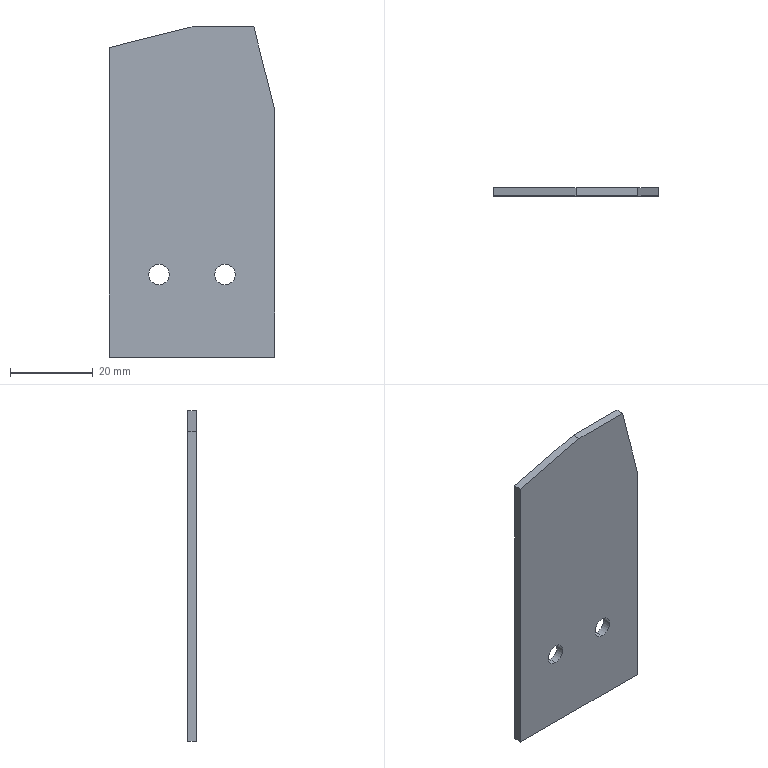Part | SolidWorks | features Chamfer 1, Cut 1, Extrusion 1 | 1 solid | 12 faces | box 40 x 2 x 80 mm | volume 6121 mm3 | plane 8 | cylinder 4 | commonest cylinder face diameters 5 x4
STEP:
#1=CARTESIAN_POINT('',(8.,2.,-22.5));
#2=VERTEX_POINT('',#1);
#3=CARTESIAN_POINT('',(8.,2.,-17.5));
#4=VERTEX_POINT('',#3);
#5=CARTESIAN_POINT('',(8.,2.,-20.));
#6=DIRECTION('',(0.,1.,0.));
#7=DIRECTION('',(0.,0.,1.));
#8=AXIS2_PLACEMENT_3D('',#5,#6,#7);
#9=CIRCLE('',#8,2.5);
#10=EDGE_CURVE('',#2,#4,#9,.T.);
#11=ORIENTED_EDGE('',*,*,#10,.T.);
#12=CARTESIAN_POINT('',(8.,0.,-17.5));
#13=VERTEX_POINT('',#12);
#14=CARTESIAN_POINT('',(8.,10.,-17.5));
#15=DIRECTION('',(0.,-1.,0.));
#16=VECTOR('',#15,1000.);
#17=LINE('',#14,#16);
#18=EDGE_CURVE('',#4,#13,#17,.T.);
#19=ORIENTED_EDGE('',*,*,#18,.T.);
#20=CARTESIAN_POINT('',(8.,0.,-22.5));
#21=VERTEX_POINT('',#20);
#22=CARTESIAN_POINT('',(8.,0.,-20.));
#23=DIRECTION('',(0.,-1.,0.));
#24=DIRECTION('',(0.,0.,-1.));
#25=AXIS2_PLACEMENT_3D('',#22,#23,#24);
#26=CIRCLE('',#25,2.5);
#27=EDGE_CURVE('',#13,#21,#26,.T.);
#28=ORIENTED_EDGE('',*,*,#27,.T.);
#29=CARTESIAN_POINT('',(8.,10.,-22.5));
#30=DIRECTION('',(0.,-1.,0.));
#31=VECTOR('',#30,1000.);
#32=LINE('',#29,#31);
#33=EDGE_CURVE('',#2,#21,#32,.T.);
#34=ORIENTED_EDGE('',*,*,#33,.F.);
#35=EDGE_LOOP('',(#11,#19,#28,#34));
#36=FACE_OUTER_BOUND('',#35,.T.);
#37=CARTESIAN_POINT('',(8.,10.,-20.));
#38=DIRECTION('',(0.,-1.,0.));
#39=DIRECTION('',(0.,0.,-1.));
#40=AXIS2_PLACEMENT_3D('',#37,#38,#39);
#41=CYLINDRICAL_SURFACE('',#40,2.5);
#42=ADVANCED_FACE('',(#36),#41,.F.);
#43=CARTESIAN_POINT('',(-8.,2.,-22.5));
#44=VERTEX_POINT('',#43);
#45=CARTESIAN_POINT('',(-8.,2.,-17.5));
#46=VERTEX_POINT('',#45);
#47=CARTESIAN_POINT('',(-8.,2.,-20.));
#48=DIRECTION('',(0.,1.,0.));
#49=DIRECTION('',(0.,0.,1.));
#50=AXIS2_PLACEMENT_3D('',#47,#48,#49);
#51=CIRCLE('',#50,2.5);
#52=EDGE_CURVE('',#44,#46,#51,.T.);
#53=ORIENTED_EDGE('',*,*,#52,.T.);
#54=CARTESIAN_POINT('',(-8.,0.,-17.5));
#55=VERTEX_POINT('',#54);
#56=CARTESIAN_POINT('',(-8.,10.,-17.5));
#57=DIRECTION('',(0.,-1.,0.));
#58=VECTOR('',#57,1000.);
#59=LINE('',#56,#58);
#60=EDGE_CURVE('',#46,#55,#59,.T.);
#61=ORIENTED_EDGE('',*,*,#60,.T.);
#62=CARTESIAN_POINT('',(-8.,0.,-22.5));
#63=VERTEX_POINT('',#62);
#64=CARTESIAN_POINT('',(-8.,0.,-20.));
#65=DIRECTION('',(0.,-1.,0.));
#66=DIRECTION('',(0.,0.,-1.));
#67=AXIS2_PLACEMENT_3D('',#64,#65,#66);
#68=CIRCLE('',#67,2.5);
#69=EDGE_CURVE('',#55,#63,#68,.T.);
#70=ORIENTED_EDGE('',*,*,#69,.T.);
#71=CARTESIAN_POINT('',(-8.,10.,-22.5));
#72=DIRECTION('',(0.,-1.,0.));
#73=VECTOR('',#72,1000.);
#74=LINE('',#71,#73);
#75=EDGE_CURVE('',#44,#63,#74,.T.);
#76=ORIENTED_EDGE('',*,*,#75,.F.);
#77=EDGE_LOOP('',(#53,#61,#70,#76));
#78=FACE_OUTER_BOUND('',#77,.T.);
#79=CARTESIAN_POINT('',(-8.,10.,-20.));
#80=DIRECTION('',(0.,-1.,0.));
#81=DIRECTION('',(0.,0.,-1.));
#82=AXIS2_PLACEMENT_3D('',#79,#80,#81);
#83=CYLINDRICAL_SURFACE('',#82,2.5);
#84=ADVANCED_FACE('',(#78),#83,.F.);
#85=CARTESIAN_POINT('',(20.,2.,20.));
#86=VERTEX_POINT('',#85);
#87=CARTESIAN_POINT('',(20.,2.,-40.));
#88=VERTEX_POINT('',#87);
#89=CARTESIAN_POINT('',(20.,2.,-40.));
#90=DIRECTION('',(0.,0.,-1.));
#91=VECTOR('',#90,1000.);
#92=LINE('',#89,#91);
#93=EDGE_CURVE('',#86,#88,#92,.T.);
#94=ORIENTED_EDGE('',*,*,#93,.F.);
#95=CARTESIAN_POINT('',(20.,0.,20.));
#96=VERTEX_POINT('',#95);
#97=CARTESIAN_POINT('',(20.,2.,20.));
#98=DIRECTION('',(0.,-1.,0.));
#99=VECTOR('',#98,1000.);
#100=LINE('',#97,#99);
#101=EDGE_CURVE('',#86,#96,#100,.T.);
#102=ORIENTED_EDGE('',*,*,#101,.T.);
#103=CARTESIAN_POINT('',(20.,0.,-40.));
#104=VERTEX_POINT('',#103);
#105=CARTESIAN_POINT('',(20.,0.,-40.));
#106=DIRECTION('',(0.,0.,-1.));
#107=VECTOR('',#106,1000.);
#108=LINE('',#105,#107);
#109=EDGE_CURVE('',#96,#104,#108,.T.);
#110=ORIENTED_EDGE('',*,*,#109,.T.);
#111=CARTESIAN_POINT('',(20.,2.,-40.));
#112=DIRECTION('',(0.,-1.,0.));
#113=VECTOR('',#112,1000.);
#114=LINE('',#111,#113);
#115=EDGE_CURVE('',#88,#104,#114,.T.);
#116=ORIENTED_EDGE('',*,*,#115,.F.);
#117=EDGE_LOOP('',(#94,#102,#110,#116));
#118=FACE_OUTER_BOUND('',#117,.T.);
#119=CARTESIAN_POINT('',(20.,2.,-40.));
#120=DIRECTION('',(-1.,0.,0.));
#121=DIRECTION('',(0.,0.,1.));
#122=AXIS2_PLACEMENT_3D('',#119,#120,#121);
#123=PLANE('',#122);
#124=ADVANCED_FACE('',(#118),#123,.F.);
#125=CARTESIAN_POINT('',(-20.,0.,-40.));
#126=VERTEX_POINT('',#125);
#127=CARTESIAN_POINT('',(-20.,0.,-40.));
#128=DIRECTION('',(-1.,0.,0.));
#129=VECTOR('',#128,1000.);
#130=LINE('',#127,#129);
#131=EDGE_CURVE('',#104,#126,#130,.T.);
#132=ORIENTED_EDGE('',*,*,#131,.T.);
#133=CARTESIAN_POINT('',(-20.,2.,-40.));
#134=VERTEX_POINT('',#133);
#135=CARTESIAN_POINT('',(-20.,2.,-40.));
#136=DIRECTION('',(0.,-1.,0.));
#137=VECTOR('',#136,1000.);
#138=LINE('',#135,#137);
#139=EDGE_CURVE('',#134,#126,#138,.T.);
#140=ORIENTED_EDGE('',*,*,#139,.F.);
#141=CARTESIAN_POINT('',(-20.,2.,-40.));
#142=DIRECTION('',(-1.,0.,0.));
#143=VECTOR('',#142,1000.);
#144=LINE('',#141,#143);
#145=EDGE_CURVE('',#88,#134,#144,.T.);
#146=ORIENTED_EDGE('',*,*,#145,.F.);
#147=ORIENTED_EDGE('',*,*,#115,.T.);
#148=EDGE_LOOP('',(#132,#140,#146,#147));
#149=FACE_OUTER_BOUND('',#148,.T.);
#150=CARTESIAN_POINT('',(-20.,2.,-40.));
#151=DIRECTION('',(0.,0.,1.));
#152=DIRECTION('',(1.,0.,0.));
#153=AXIS2_PLACEMENT_3D('',#150,#151,#152);
#154=PLANE('',#153);
#155=ADVANCED_FACE('',(#149),#154,.F.);
#156=CARTESIAN_POINT('',(-20.,0.,35.));
#157=VERTEX_POINT('',#156);
#158=CARTESIAN_POINT('',(-20.,0.,-40.));
#159=DIRECTION('',(0.,0.,1.));
#160=VECTOR('',#159,1000.);
#161=LINE('',#158,#160);
#162=EDGE_CURVE('',#126,#157,#161,.T.);
#163=ORIENTED_EDGE('',*,*,#162,.T.);
#164=CARTESIAN_POINT('',(-20.,2.,35.));
#165=VERTEX_POINT('',#164);
#166=CARTESIAN_POINT('',(-20.,2.,35.));
#167=DIRECTION('',(0.,1.,0.));
#168=VECTOR('',#167,1000.);
#169=LINE('',#166,#168);
#170=EDGE_CURVE('',#157,#165,#169,.T.);
#171=ORIENTED_EDGE('',*,*,#170,.T.);
#172=CARTESIAN_POINT('',(-20.,2.,-40.));
#173=DIRECTION('',(0.,0.,1.));
#174=VECTOR('',#173,1000.);
#175=LINE('',#172,#174);
#176=EDGE_CURVE('',#134,#165,#175,.T.);
#177=ORIENTED_EDGE('',*,*,#176,.F.);
#178=ORIENTED_EDGE('',*,*,#139,.T.);
#179=EDGE_LOOP('',(#163,#171,#177,#178));
#180=FACE_OUTER_BOUND('',#179,.T.);
#181=CARTESIAN_POINT('',(-20.,2.,-40.));
#182=DIRECTION('',(1.,0.,0.));
#183=DIRECTION('',(0.,0.,-1.));
#184=AXIS2_PLACEMENT_3D('',#181,#182,#183);
#185=PLANE('',#184);
#186=ADVANCED_FACE('',(#180),#185,.F.);
#187=CARTESIAN_POINT('',(0.,0.,40.));
#188=VERTEX_POINT('',#187);
#189=CARTESIAN_POINT('',(15.,0.,40.));
#190=VERTEX_POINT('',#189);
#191=CARTESIAN_POINT('',(-20.,0.,40.));
#192=DIRECTION('',(1.,0.,0.));
#193=VECTOR('',#192,1000.);
#194=LINE('',#191,#193);
#195=EDGE_CURVE('',#188,#190,#194,.T.);
#196=ORIENTED_EDGE('',*,*,#195,.T.);
#197=CARTESIAN_POINT('',(15.,2.,40.));
#198=VERTEX_POINT('',#197);
#199=CARTESIAN_POINT('',(15.,2.,40.));
#200=DIRECTION('',(0.,1.,0.));
#201=VECTOR('',#200,1000.);
#202=LINE('',#199,#201);
#203=EDGE_CURVE('',#190,#198,#202,.T.);
#204=ORIENTED_EDGE('',*,*,#203,.T.);
#205=CARTESIAN_POINT('',(0.,2.,40.));
#206=VERTEX_POINT('',#205);
#207=CARTESIAN_POINT('',(-20.,2.,40.));
#208=DIRECTION('',(1.,0.,0.));
#209=VECTOR('',#208,1000.);
#210=LINE('',#207,#209);
#211=EDGE_CURVE('',#206,#198,#210,.T.);
#212=ORIENTED_EDGE('',*,*,#211,.F.);
#213=CARTESIAN_POINT('',(0.,2.,40.));
#214=DIRECTION('',(0.,-1.,0.));
#215=VECTOR('',#214,1000.);
#216=LINE('',#213,#215);
#217=EDGE_CURVE('',#206,#188,#216,.T.);
#218=ORIENTED_EDGE('',*,*,#217,.T.);
#219=EDGE_LOOP('',(#196,#204,#212,#218));
#220=FACE_OUTER_BOUND('',#219,.T.);
#221=CARTESIAN_POINT('',(-20.,2.,40.));
#222=DIRECTION('',(0.,0.,-1.));
#223=DIRECTION('',(-1.,0.,0.));
#224=AXIS2_PLACEMENT_3D('',#221,#222,#223);
#225=PLANE('',#224);
#226=ADVANCED_FACE('',(#220),#225,.F.);
#227=ORIENTED_EDGE('',*,*,#10,.F.);
#228=CARTESIAN_POINT('',(8.,2.,-20.));
#229=DIRECTION('',(0.,1.,0.));
#230=DIRECTION('',(0.,0.,1.));
#231=AXIS2_PLACEMENT_3D('',#228,#229,#230);
#232=CIRCLE('',#231,2.5);
#233=EDGE_CURVE('',#4,#2,#232,.T.);
#234=ORIENTED_EDGE('',*,*,#233,.F.);
#235=EDGE_LOOP('',(#227,#234));
#236=FACE_BOUND('',#235,.T.);
#237=ORIENTED_EDGE('',*,*,#52,.F.);
#238=CARTESIAN_POINT('',(-8.,2.,-20.));
#239=DIRECTION('',(0.,1.,0.));
#240=DIRECTION('',(0.,0.,1.));
#241=AXIS2_PLACEMENT_3D('',#238,#239,#240);
#242=CIRCLE('',#241,2.5);
#243=EDGE_CURVE('',#46,#44,#242,.T.);
#244=ORIENTED_EDGE('',*,*,#243,.F.);
#245=EDGE_LOOP('',(#237,#244));
#246=FACE_BOUND('',#245,.T.);
#247=ORIENTED_EDGE('',*,*,#211,.T.);
#248=CARTESIAN_POINT('',(23.529,2.,5.882));
#249=DIRECTION('',(0.2425,0.,-0.9701));
#250=VECTOR('',#249,1000.);
#251=LINE('',#248,#250);
#252=EDGE_CURVE('',#198,#86,#251,.T.);
#253=ORIENTED_EDGE('',*,*,#252,.T.);
#254=ORIENTED_EDGE('',*,*,#93,.T.);
#255=ORIENTED_EDGE('',*,*,#145,.T.);
#256=ORIENTED_EDGE('',*,*,#176,.T.);
#257=CARTESIAN_POINT('',(-9.412,2.,37.647));
#258=DIRECTION('',(0.9701,0.,0.2425));
#259=VECTOR('',#258,1000.);
#260=LINE('',#257,#259);
#261=EDGE_CURVE('',#165,#206,#260,.T.);
#262=ORIENTED_EDGE('',*,*,#261,.T.);
#263=EDGE_LOOP('',(#247,#253,#254,#255,#256,#262));
#264=FACE_OUTER_BOUND('',#263,.T.);
#265=CARTESIAN_POINT('',(0.,2.,0.));
#266=DIRECTION('',(0.,1.,0.));
#267=DIRECTION('',(0.,0.,1.));
#268=AXIS2_PLACEMENT_3D('',#265,#266,#267);
#269=PLANE('',#268);
#270=ADVANCED_FACE('',(#236,#246,#264),#269,.T.);
#271=CARTESIAN_POINT('',(8.,0.,-20.));
#272=DIRECTION('',(0.,-1.,0.));
#273=DIRECTION('',(0.,0.,-1.));
#274=AXIS2_PLACEMENT_3D('',#271,#272,#273);
#275=CIRCLE('',#274,2.5);
#276=EDGE_CURVE('',#21,#13,#275,.T.);
#277=ORIENTED_EDGE('',*,*,#276,.F.);
#278=ORIENTED_EDGE('',*,*,#27,.F.);
#279=EDGE_LOOP('',(#277,#278));
#280=FACE_BOUND('',#279,.T.);
#281=CARTESIAN_POINT('',(-8.,0.,-20.));
#282=DIRECTION('',(0.,-1.,0.));
#283=DIRECTION('',(0.,0.,-1.));
#284=AXIS2_PLACEMENT_3D('',#281,#282,#283);
#285=CIRCLE('',#284,2.5);
#286=EDGE_CURVE('',#63,#55,#285,.T.);
#287=ORIENTED_EDGE('',*,*,#286,.F.);
#288=ORIENTED_EDGE('',*,*,#69,.F.);
#289=EDGE_LOOP('',(#287,#288));
#290=FACE_BOUND('',#289,.T.);
#291=ORIENTED_EDGE('',*,*,#109,.F.);
#292=CARTESIAN_POINT('',(20.,0.,20.));
#293=DIRECTION('',(-0.2425,0.,0.9701));
#294=VECTOR('',#293,1000.);
#295=LINE('',#292,#294);
#296=EDGE_CURVE('',#96,#190,#295,.T.);
#297=ORIENTED_EDGE('',*,*,#296,.T.);
#298=ORIENTED_EDGE('',*,*,#195,.F.);
#299=CARTESIAN_POINT('',(0.,0.,40.));
#300=DIRECTION('',(-0.9701,0.,-0.2425));
#301=VECTOR('',#300,1000.);
#302=LINE('',#299,#301);
#303=EDGE_CURVE('',#188,#157,#302,.T.);
#304=ORIENTED_EDGE('',*,*,#303,.T.);
#305=ORIENTED_EDGE('',*,*,#162,.F.);
#306=ORIENTED_EDGE('',*,*,#131,.F.);
#307=EDGE_LOOP('',(#291,#297,#298,#304,#305,#306));
#308=FACE_OUTER_BOUND('',#307,.T.);
#309=CARTESIAN_POINT('',(0.,0.,0.));
#310=DIRECTION('',(0.,1.,0.));
#311=DIRECTION('',(0.,0.,1.));
#312=AXIS2_PLACEMENT_3D('',#309,#310,#311);
#313=PLANE('',#312);
#314=ADVANCED_FACE('',(#280,#290,#308),#313,.F.);
#315=ORIENTED_EDGE('',*,*,#60,.F.);
#316=ORIENTED_EDGE('',*,*,#243,.T.);
#317=ORIENTED_EDGE('',*,*,#75,.T.);
#318=ORIENTED_EDGE('',*,*,#286,.T.);
#319=EDGE_LOOP('',(#315,#316,#317,#318));
#320=FACE_OUTER_BOUND('',#319,.T.);
#321=CARTESIAN_POINT('',(-8.,10.,-20.));
#322=DIRECTION('',(0.,-1.,0.));
#323=DIRECTION('',(0.,0.,-1.));
#324=AXIS2_PLACEMENT_3D('',#321,#322,#323);
#325=CYLINDRICAL_SURFACE('',#324,2.5);
#326=ADVANCED_FACE('',(#320),#325,.F.);
#327=ORIENTED_EDGE('',*,*,#18,.F.);
#328=ORIENTED_EDGE('',*,*,#233,.T.);
#329=ORIENTED_EDGE('',*,*,#33,.T.);
#330=ORIENTED_EDGE('',*,*,#276,.T.);
#331=EDGE_LOOP('',(#327,#328,#329,#330));
#332=FACE_OUTER_BOUND('',#331,.T.);
#333=CARTESIAN_POINT('',(8.,10.,-20.));
#334=DIRECTION('',(0.,-1.,0.));
#335=DIRECTION('',(0.,0.,-1.));
#336=AXIS2_PLACEMENT_3D('',#333,#334,#335);
#337=CYLINDRICAL_SURFACE('',#336,2.5);
#338=ADVANCED_FACE('',(#332),#337,.F.);
#339=ORIENTED_EDGE('',*,*,#252,.F.);
#340=ORIENTED_EDGE('',*,*,#203,.F.);
#341=ORIENTED_EDGE('',*,*,#296,.F.);
#342=ORIENTED_EDGE('',*,*,#101,.F.);
#343=EDGE_LOOP('',(#339,#340,#341,#342));
#344=FACE_OUTER_BOUND('',#343,.T.);
#345=CARTESIAN_POINT('',(20.,2.,20.));
#346=DIRECTION('',(-0.9701,0.,-0.2425));
#347=DIRECTION('',(0.,-1.,0.));
#348=AXIS2_PLACEMENT_3D('',#345,#346,#347);
#349=PLANE('',#348);
#350=ADVANCED_FACE('',(#344),#349,.F.);
#351=ORIENTED_EDGE('',*,*,#261,.F.);
#352=ORIENTED_EDGE('',*,*,#170,.F.);
#353=ORIENTED_EDGE('',*,*,#303,.F.);
#354=ORIENTED_EDGE('',*,*,#217,.F.);
#355=EDGE_LOOP('',(#351,#352,#353,#354));
#356=FACE_OUTER_BOUND('',#355,.T.);
#357=CARTESIAN_POINT('',(0.,2.,40.));
#358=DIRECTION('',(0.2425,0.,-0.9701));
#359=DIRECTION('',(0.,-1.,0.));
#360=AXIS2_PLACEMENT_3D('',#357,#358,#359);
#361=PLANE('',#360);
#362=ADVANCED_FACE('',(#356),#361,.F.);
#363=CLOSED_SHELL('',(#42,#84,#124,#155,#186,#226,#270,#314,#326,#338,#350,#362));
#364=MANIFOLD_SOLID_BREP('',#363);
#365=CARTESIAN_POINT('',(0.,0.,0.));
#366=DIRECTION('',(0.,0.,1.));
#367=DIRECTION('',(1.,0.,0.));
#368=AXIS2_PLACEMENT_3D('',#365,#366,#367);
#369=(LENGTH_UNIT()NAMED_UNIT(*)SI_UNIT(.MILLI.,.METRE.));
#370=UNCERTAINTY_MEASURE_WITH_UNIT(LENGTH_MEASURE(0.00001),#369,'','');
#371=(NAMED_UNIT(*)PLANE_ANGLE_UNIT()SI_UNIT($,.RADIAN.));
#372=(NAMED_UNIT(*)SI_UNIT($,.STERADIAN.)SOLID_ANGLE_UNIT());
#373=(GEOMETRIC_REPRESENTATION_CONTEXT(3)GLOBAL_UNCERTAINTY_ASSIGNED_CONTEXT((#370))GLOBAL_UNIT_ASSIGNED_CONTEXT((#369,#371,#372))REPRESENTATION_CONTEXT('',''));
#374=ADVANCED_BREP_SHAPE_REPRESENTATION('',(#364,#368),#373);